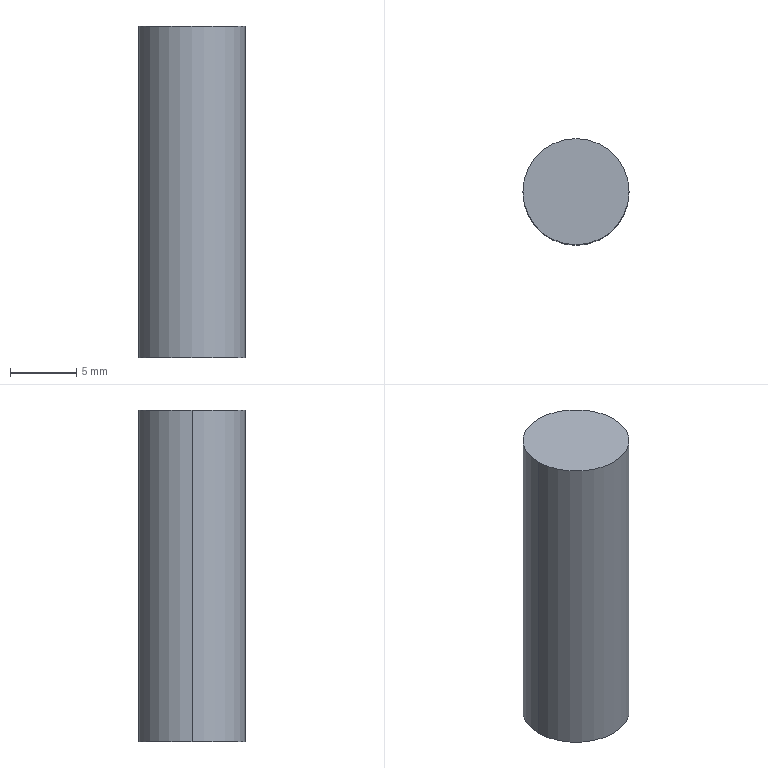Part | SolidWorks | features Extrusion 1 | 1 solid | 4 faces | box 8 x 8 x 25 mm | volume 1257 mm3 | cylinder 2 | plane 2 | commonest cylinder face diameters 8 x2
STEP:
#1=CARTESIAN_POINT('',(4.,0.,25.));
#2=VERTEX_POINT('',#1);
#3=CARTESIAN_POINT('',(-4.,0.,25.));
#4=VERTEX_POINT('',#3);
#5=CARTESIAN_POINT('',(0.,0.,25.));
#6=DIRECTION('',(0.,0.,1.));
#7=DIRECTION('',(1.,0.,0.));
#8=AXIS2_PLACEMENT_3D('',#5,#6,#7);
#9=CIRCLE('',#8,4.);
#10=EDGE_CURVE('',#2,#4,#9,.T.);
#11=ORIENTED_EDGE('',*,*,#10,.F.);
#12=CARTESIAN_POINT('',(4.,0.,0.));
#13=VERTEX_POINT('',#12);
#14=CARTESIAN_POINT('',(4.,0.,25.));
#15=DIRECTION('',(0.,0.,-1.));
#16=VECTOR('',#15,1000.);
#17=LINE('',#14,#16);
#18=EDGE_CURVE('',#2,#13,#17,.T.);
#19=ORIENTED_EDGE('',*,*,#18,.T.);
#20=CARTESIAN_POINT('',(-4.,0.,0.));
#21=VERTEX_POINT('',#20);
#22=CARTESIAN_POINT('',(0.,0.,0.));
#23=DIRECTION('',(0.,0.,1.));
#24=DIRECTION('',(1.,0.,0.));
#25=AXIS2_PLACEMENT_3D('',#22,#23,#24);
#26=CIRCLE('',#25,4.);
#27=EDGE_CURVE('',#13,#21,#26,.T.);
#28=ORIENTED_EDGE('',*,*,#27,.T.);
#29=CARTESIAN_POINT('',(-4.,0.,25.));
#30=DIRECTION('',(0.,0.,-1.));
#31=VECTOR('',#30,1000.);
#32=LINE('',#29,#31);
#33=EDGE_CURVE('',#4,#21,#32,.T.);
#34=ORIENTED_EDGE('',*,*,#33,.F.);
#35=EDGE_LOOP('',(#11,#19,#28,#34));
#36=FACE_OUTER_BOUND('',#35,.T.);
#37=CARTESIAN_POINT('',(0.,0.,25.));
#38=DIRECTION('',(0.,0.,-1.));
#39=DIRECTION('',(-1.,0.,0.));
#40=AXIS2_PLACEMENT_3D('',#37,#38,#39);
#41=CYLINDRICAL_SURFACE('',#40,4.);
#42=ADVANCED_FACE('',(#36),#41,.T.);
#43=ORIENTED_EDGE('',*,*,#18,.F.);
#44=CARTESIAN_POINT('',(0.,0.,25.));
#45=DIRECTION('',(0.,0.,1.));
#46=DIRECTION('',(1.,0.,0.));
#47=AXIS2_PLACEMENT_3D('',#44,#45,#46);
#48=CIRCLE('',#47,4.);
#49=EDGE_CURVE('',#4,#2,#48,.T.);
#50=ORIENTED_EDGE('',*,*,#49,.F.);
#51=ORIENTED_EDGE('',*,*,#33,.T.);
#52=CARTESIAN_POINT('',(0.,0.,0.));
#53=DIRECTION('',(0.,0.,1.));
#54=DIRECTION('',(1.,0.,0.));
#55=AXIS2_PLACEMENT_3D('',#52,#53,#54);
#56=CIRCLE('',#55,4.);
#57=EDGE_CURVE('',#21,#13,#56,.T.);
#58=ORIENTED_EDGE('',*,*,#57,.T.);
#59=EDGE_LOOP('',(#43,#50,#51,#58));
#60=FACE_OUTER_BOUND('',#59,.T.);
#61=CARTESIAN_POINT('',(0.,0.,25.));
#62=DIRECTION('',(0.,0.,-1.));
#63=DIRECTION('',(-1.,0.,0.));
#64=AXIS2_PLACEMENT_3D('',#61,#62,#63);
#65=CYLINDRICAL_SURFACE('',#64,4.);
#66=ADVANCED_FACE('',(#60),#65,.T.);
#67=ORIENTED_EDGE('',*,*,#49,.T.);
#68=ORIENTED_EDGE('',*,*,#10,.T.);
#69=EDGE_LOOP('',(#67,#68));
#70=FACE_OUTER_BOUND('',#69,.T.);
#71=CARTESIAN_POINT('',(0.,0.,25.));
#72=DIRECTION('',(0.,0.,1.));
#73=DIRECTION('',(1.,0.,0.));
#74=AXIS2_PLACEMENT_3D('',#71,#72,#73);
#75=PLANE('',#74);
#76=ADVANCED_FACE('',(#70),#75,.T.);
#77=ORIENTED_EDGE('',*,*,#57,.F.);
#78=ORIENTED_EDGE('',*,*,#27,.F.);
#79=EDGE_LOOP('',(#77,#78));
#80=FACE_OUTER_BOUND('',#79,.T.);
#81=CARTESIAN_POINT('',(0.,0.,0.));
#82=DIRECTION('',(0.,0.,1.));
#83=DIRECTION('',(1.,0.,0.));
#84=AXIS2_PLACEMENT_3D('',#81,#82,#83);
#85=PLANE('',#84);
#86=ADVANCED_FACE('',(#80),#85,.F.);
#87=CLOSED_SHELL('',(#42,#66,#76,#86));
#88=MANIFOLD_SOLID_BREP('',#87);
#89=CARTESIAN_POINT('',(0.,0.,0.));
#90=DIRECTION('',(0.,0.,1.));
#91=DIRECTION('',(1.,0.,0.));
#92=AXIS2_PLACEMENT_3D('',#89,#90,#91);
#93=(LENGTH_UNIT()NAMED_UNIT(*)SI_UNIT(.MILLI.,.METRE.));
#94=UNCERTAINTY_MEASURE_WITH_UNIT(LENGTH_MEASURE(0.00001),#93,'','');
#95=(NAMED_UNIT(*)PLANE_ANGLE_UNIT()SI_UNIT($,.RADIAN.));
#96=(NAMED_UNIT(*)SI_UNIT($,.STERADIAN.)SOLID_ANGLE_UNIT());
#97=(GEOMETRIC_REPRESENTATION_CONTEXT(3)GLOBAL_UNCERTAINTY_ASSIGNED_CONTEXT((#94))GLOBAL_UNIT_ASSIGNED_CONTEXT((#93,#95,#96))REPRESENTATION_CONTEXT('',''));
#98=ADVANCED_BREP_SHAPE_REPRESENTATION('',(#88,#92),#97);